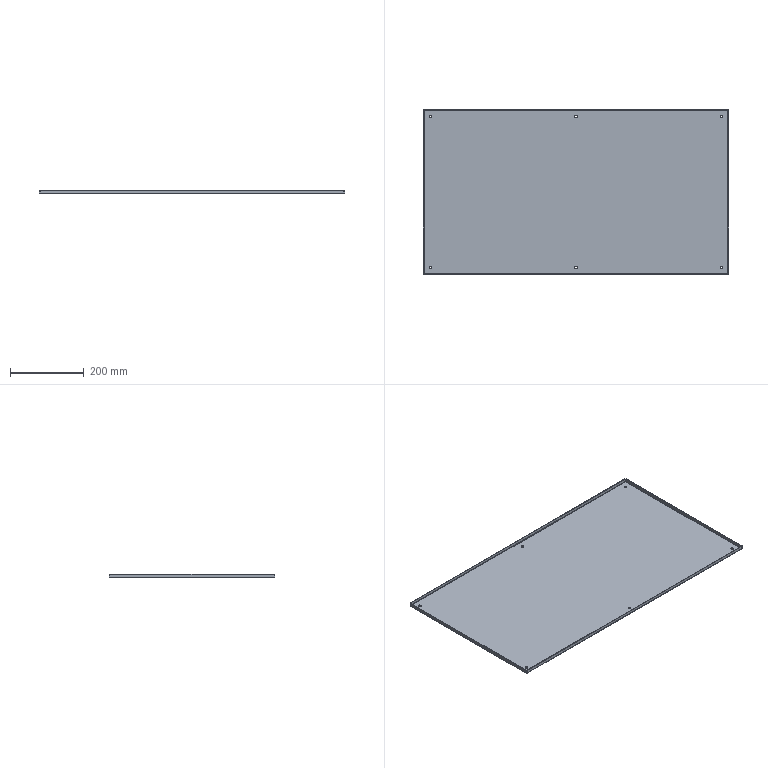Part | SolidWorks | features BaseBody 1 | 1 solid | 50 faces | box 830 x 450 x 10 mm | volume 589856 mm3 | plane 22 | cylinder 20 | spline 8 | commonest cylinder face diameters 7 x12 1.473 x4 4.473 x4